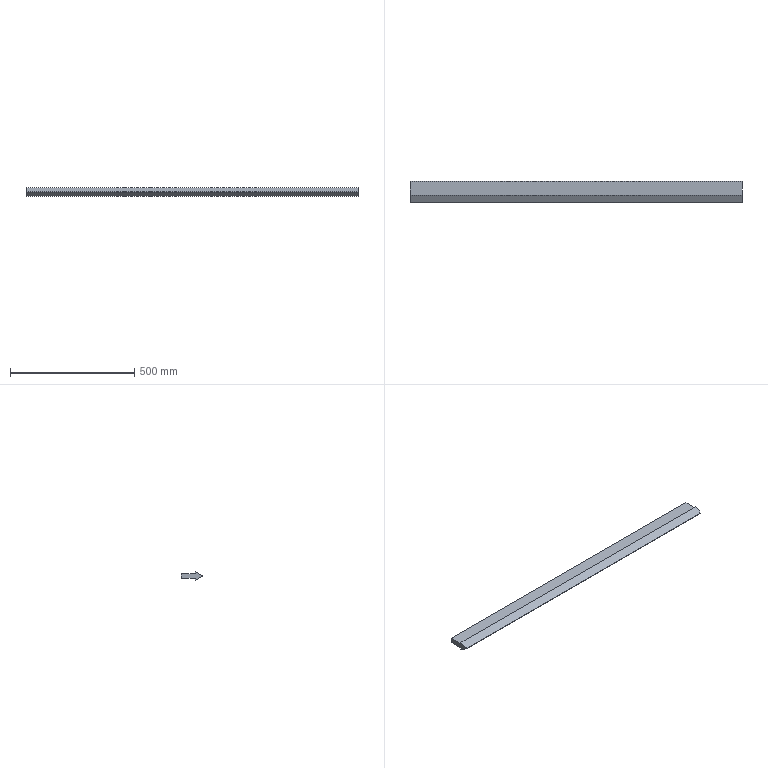Part | SolidWorks | features Extrusion 1, Fillet 1, HoleWzd 1 | 1 solid | 34 faces | box 1337 x 85 x 34.641 mm | volume 2189424 mm3 | cylinder 13 | cone 12 | plane 9 | commonest cylinder face diameters 5 x12 2 x1
STEP:
#1=CARTESIAN_POINT('',(20.,71.,-2.5));
#2=VERTEX_POINT('',#1);
#3=CARTESIAN_POINT('',(20.,71.,2.5));
#4=VERTEX_POINT('',#3);
#5=CARTESIAN_POINT('',(20.,71.,0.));
#6=DIRECTION('',(0.,1.,0.));
#7=DIRECTION('',(0.,0.,1.));
#8=AXIS2_PLACEMENT_3D('',#5,#6,#7);
#9=CIRCLE('',#8,2.5);
#10=EDGE_CURVE('',#2,#4,#9,.T.);
#11=ORIENTED_EDGE('',*,*,#10,.F.);
#12=CARTESIAN_POINT('',(20.,86.,-2.5));
#13=VERTEX_POINT('',#12);
#14=CARTESIAN_POINT('',(20.,86.,-2.5));
#15=DIRECTION('',(0.,1.,0.));
#16=VECTOR('',#15,1000.);
#17=LINE('',#14,#16);
#18=EDGE_CURVE('',#2,#13,#17,.T.);
#19=ORIENTED_EDGE('',*,*,#18,.T.);
#20=CARTESIAN_POINT('',(20.,86.,2.5));
#21=VERTEX_POINT('',#20);
#22=CARTESIAN_POINT('',(20.,86.,0.));
#23=DIRECTION('',(0.,1.,0.));
#24=DIRECTION('',(0.,0.,1.));
#25=AXIS2_PLACEMENT_3D('',#22,#23,#24);
#26=CIRCLE('',#25,2.5);
#27=EDGE_CURVE('',#13,#21,#26,.T.);
#28=ORIENTED_EDGE('',*,*,#27,.T.);
#29=CARTESIAN_POINT('',(20.,86.,2.5));
#30=DIRECTION('',(0.,1.,0.));
#31=VECTOR('',#30,1000.);
#32=LINE('',#29,#31);
#33=EDGE_CURVE('',#4,#21,#32,.T.);
#34=ORIENTED_EDGE('',*,*,#33,.F.);
#35=EDGE_LOOP('',(#11,#19,#28,#34));
#36=FACE_OUTER_BOUND('',#35,.T.);
#37=CARTESIAN_POINT('',(20.,86.,0.));
#38=DIRECTION('',(0.,1.,0.));
#39=DIRECTION('',(0.,0.,1.));
#40=AXIS2_PLACEMENT_3D('',#37,#38,#39);
#41=CYLINDRICAL_SURFACE('',#40,2.5);
#42=ADVANCED_FACE('',(#36),#41,.F.);
#43=CARTESIAN_POINT('',(20.,69.498,0.));
#44=VERTEX_POINT('',#43);
#45=CARTESIAN_POINT('',(20.,71.,2.5));
#46=DIRECTION('',(0.,0.515,0.8572));
#47=VECTOR('',#46,1000.);
#48=LINE('',#45,#47);
#49=EDGE_CURVE('',#44,#4,#48,.T.);
#50=ORIENTED_EDGE('',*,*,#49,.F.);
#51=CARTESIAN_POINT('',(20.,71.,-2.5));
#52=DIRECTION('',(0.,0.515,-0.8572));
#53=VECTOR('',#52,1000.);
#54=LINE('',#51,#53);
#55=EDGE_CURVE('',#44,#2,#54,.T.);
#56=ORIENTED_EDGE('',*,*,#55,.T.);
#57=ORIENTED_EDGE('',*,*,#10,.T.);
#58=EDGE_LOOP('',(#50,#56,#57));
#59=FACE_OUTER_BOUND('',#58,.T.);
#60=CARTESIAN_POINT('',(20.,71.,0.));
#61=DIRECTION('',(0.,1.,0.));
#62=DIRECTION('',(0.,0.,1.));
#63=AXIS2_PLACEMENT_3D('',#60,#61,#62);
#64=CONICAL_SURFACE('',#63,2.5,1.03);
#65=ADVANCED_FACE('',(#59),#64,.F.);
#66=CARTESIAN_POINT('',(45.,71.,-2.5));
#67=VERTEX_POINT('',#66);
#68=CARTESIAN_POINT('',(45.,71.,2.5));
#69=VERTEX_POINT('',#68);
#70=CARTESIAN_POINT('',(45.,71.,0.));
#71=DIRECTION('',(0.,1.,0.));
#72=DIRECTION('',(0.,0.,1.));
#73=AXIS2_PLACEMENT_3D('',#70,#71,#72);
#74=CIRCLE('',#73,2.5);
#75=EDGE_CURVE('',#67,#69,#74,.T.);
#76=ORIENTED_EDGE('',*,*,#75,.F.);
#77=CARTESIAN_POINT('',(45.,86.,-2.5));
#78=VERTEX_POINT('',#77);
#79=CARTESIAN_POINT('',(45.,86.,-2.5));
#80=DIRECTION('',(0.,1.,0.));
#81=VECTOR('',#80,1000.);
#82=LINE('',#79,#81);
#83=EDGE_CURVE('',#67,#78,#82,.T.);
#84=ORIENTED_EDGE('',*,*,#83,.T.);
#85=CARTESIAN_POINT('',(45.,86.,2.5));
#86=VERTEX_POINT('',#85);
#87=CARTESIAN_POINT('',(45.,86.,0.));
#88=DIRECTION('',(0.,1.,0.));
#89=DIRECTION('',(0.,0.,1.));
#90=AXIS2_PLACEMENT_3D('',#87,#88,#89);
#91=CIRCLE('',#90,2.5);
#92=EDGE_CURVE('',#78,#86,#91,.T.);
#93=ORIENTED_EDGE('',*,*,#92,.T.);
#94=CARTESIAN_POINT('',(45.,86.,2.5));
#95=DIRECTION('',(0.,1.,0.));
#96=VECTOR('',#95,1000.);
#97=LINE('',#94,#96);
#98=EDGE_CURVE('',#69,#86,#97,.T.);
#99=ORIENTED_EDGE('',*,*,#98,.F.);
#100=EDGE_LOOP('',(#76,#84,#93,#99));
#101=FACE_OUTER_BOUND('',#100,.T.);
#102=CARTESIAN_POINT('',(45.,86.,0.));
#103=DIRECTION('',(0.,1.,0.));
#104=DIRECTION('',(0.,0.,1.));
#105=AXIS2_PLACEMENT_3D('',#102,#103,#104);
#106=CYLINDRICAL_SURFACE('',#105,2.5);
#107=ADVANCED_FACE('',(#101),#106,.F.);
#108=CARTESIAN_POINT('',(45.,69.498,0.));
#109=VERTEX_POINT('',#108);
#110=CARTESIAN_POINT('',(45.,71.,2.5));
#111=DIRECTION('',(0.,0.515,0.8572));
#112=VECTOR('',#111,1000.);
#113=LINE('',#110,#112);
#114=EDGE_CURVE('',#109,#69,#113,.T.);
#115=ORIENTED_EDGE('',*,*,#114,.F.);
#116=CARTESIAN_POINT('',(45.,71.,-2.5));
#117=DIRECTION('',(0.,0.515,-0.8572));
#118=VECTOR('',#117,1000.);
#119=LINE('',#116,#118);
#120=EDGE_CURVE('',#109,#67,#119,.T.);
#121=ORIENTED_EDGE('',*,*,#120,.T.);
#122=ORIENTED_EDGE('',*,*,#75,.T.);
#123=EDGE_LOOP('',(#115,#121,#122));
#124=FACE_OUTER_BOUND('',#123,.T.);
#125=CARTESIAN_POINT('',(45.,71.,0.));
#126=DIRECTION('',(0.,1.,0.));
#127=DIRECTION('',(0.,0.,1.));
#128=AXIS2_PLACEMENT_3D('',#125,#126,#127);
#129=CONICAL_SURFACE('',#128,2.5,1.03);
#130=ADVANCED_FACE('',(#124),#129,.F.);
#131=CARTESIAN_POINT('',(70.,71.,-2.5));
#132=VERTEX_POINT('',#131);
#133=CARTESIAN_POINT('',(70.,71.,2.5));
#134=VERTEX_POINT('',#133);
#135=CARTESIAN_POINT('',(70.,71.,0.));
#136=DIRECTION('',(0.,1.,0.));
#137=DIRECTION('',(0.,0.,1.));
#138=AXIS2_PLACEMENT_3D('',#135,#136,#137);
#139=CIRCLE('',#138,2.5);
#140=EDGE_CURVE('',#132,#134,#139,.T.);
#141=ORIENTED_EDGE('',*,*,#140,.F.);
#142=CARTESIAN_POINT('',(70.,86.,-2.5));
#143=VERTEX_POINT('',#142);
#144=CARTESIAN_POINT('',(70.,86.,-2.5));
#145=DIRECTION('',(0.,1.,0.));
#146=VECTOR('',#145,1000.);
#147=LINE('',#144,#146);
#148=EDGE_CURVE('',#132,#143,#147,.T.);
#149=ORIENTED_EDGE('',*,*,#148,.T.);
#150=CARTESIAN_POINT('',(70.,86.,2.5));
#151=VERTEX_POINT('',#150);
#152=CARTESIAN_POINT('',(70.,86.,0.));
#153=DIRECTION('',(0.,1.,0.));
#154=DIRECTION('',(0.,0.,1.));
#155=AXIS2_PLACEMENT_3D('',#152,#153,#154);
#156=CIRCLE('',#155,2.5);
#157=EDGE_CURVE('',#143,#151,#156,.T.);
#158=ORIENTED_EDGE('',*,*,#157,.T.);
#159=CARTESIAN_POINT('',(70.,86.,2.5));
#160=DIRECTION('',(0.,1.,0.));
#161=VECTOR('',#160,1000.);
#162=LINE('',#159,#161);
#163=EDGE_CURVE('',#134,#151,#162,.T.);
#164=ORIENTED_EDGE('',*,*,#163,.F.);
#165=EDGE_LOOP('',(#141,#149,#158,#164));
#166=FACE_OUTER_BOUND('',#165,.T.);
#167=CARTESIAN_POINT('',(70.,86.,0.));
#168=DIRECTION('',(0.,1.,0.));
#169=DIRECTION('',(0.,0.,1.));
#170=AXIS2_PLACEMENT_3D('',#167,#168,#169);
#171=CYLINDRICAL_SURFACE('',#170,2.5);
#172=ADVANCED_FACE('',(#166),#171,.F.);
#173=CARTESIAN_POINT('',(70.,69.498,0.));
#174=VERTEX_POINT('',#173);
#175=CARTESIAN_POINT('',(70.,71.,2.5));
#176=DIRECTION('',(0.,0.515,0.8572));
#177=VECTOR('',#176,1000.);
#178=LINE('',#175,#177);
#179=EDGE_CURVE('',#174,#134,#178,.T.);
#180=ORIENTED_EDGE('',*,*,#179,.F.);
#181=CARTESIAN_POINT('',(70.,71.,-2.5));
#182=DIRECTION('',(0.,0.515,-0.8572));
#183=VECTOR('',#182,1000.);
#184=LINE('',#181,#183);
#185=EDGE_CURVE('',#174,#132,#184,.T.);
#186=ORIENTED_EDGE('',*,*,#185,.T.);
#187=ORIENTED_EDGE('',*,*,#140,.T.);
#188=EDGE_LOOP('',(#180,#186,#187));
#189=FACE_OUTER_BOUND('',#188,.T.);
#190=CARTESIAN_POINT('',(70.,71.,0.));
#191=DIRECTION('',(0.,1.,0.));
#192=DIRECTION('',(0.,0.,1.));
#193=AXIS2_PLACEMENT_3D('',#190,#191,#192);
#194=CONICAL_SURFACE('',#193,2.5,1.03);
#195=ADVANCED_FACE('',(#189),#194,.F.);
#196=CARTESIAN_POINT('',(1317.,71.,-2.5));
#197=VERTEX_POINT('',#196);
#198=CARTESIAN_POINT('',(1317.,71.,2.5));
#199=VERTEX_POINT('',#198);
#200=CARTESIAN_POINT('',(1317.,71.,0.));
#201=DIRECTION('',(0.,1.,0.));
#202=DIRECTION('',(0.,0.,1.));
#203=AXIS2_PLACEMENT_3D('',#200,#201,#202);
#204=CIRCLE('',#203,2.5);
#205=EDGE_CURVE('',#197,#199,#204,.T.);
#206=ORIENTED_EDGE('',*,*,#205,.F.);
#207=CARTESIAN_POINT('',(1317.,86.,-2.5));
#208=VERTEX_POINT('',#207);
#209=CARTESIAN_POINT('',(1317.,86.,-2.5));
#210=DIRECTION('',(0.,1.,0.));
#211=VECTOR('',#210,1000.);
#212=LINE('',#209,#211);
#213=EDGE_CURVE('',#197,#208,#212,.T.);
#214=ORIENTED_EDGE('',*,*,#213,.T.);
#215=CARTESIAN_POINT('',(1317.,86.,2.5));
#216=VERTEX_POINT('',#215);
#217=CARTESIAN_POINT('',(1317.,86.,0.));
#218=DIRECTION('',(0.,1.,0.));
#219=DIRECTION('',(0.,0.,1.));
#220=AXIS2_PLACEMENT_3D('',#217,#218,#219);
#221=CIRCLE('',#220,2.5);
#222=EDGE_CURVE('',#208,#216,#221,.T.);
#223=ORIENTED_EDGE('',*,*,#222,.T.);
#224=CARTESIAN_POINT('',(1317.,86.,2.5));
#225=DIRECTION('',(0.,1.,0.));
#226=VECTOR('',#225,1000.);
#227=LINE('',#224,#226);
#228=EDGE_CURVE('',#199,#216,#227,.T.);
#229=ORIENTED_EDGE('',*,*,#228,.F.);
#230=EDGE_LOOP('',(#206,#214,#223,#229));
#231=FACE_OUTER_BOUND('',#230,.T.);
#232=CARTESIAN_POINT('',(1317.,86.,0.));
#233=DIRECTION('',(0.,1.,0.));
#234=DIRECTION('',(0.,0.,1.));
#235=AXIS2_PLACEMENT_3D('',#232,#233,#234);
#236=CYLINDRICAL_SURFACE('',#235,2.5);
#237=ADVANCED_FACE('',(#231),#236,.F.);
#238=CARTESIAN_POINT('',(1317.,69.498,0.));
#239=VERTEX_POINT('',#238);
#240=CARTESIAN_POINT('',(1317.,71.,2.5));
#241=DIRECTION('',(0.,0.515,0.8572));
#242=VECTOR('',#241,1000.);
#243=LINE('',#240,#242);
#244=EDGE_CURVE('',#239,#199,#243,.T.);
#245=ORIENTED_EDGE('',*,*,#244,.F.);
#246=CARTESIAN_POINT('',(1317.,71.,-2.5));
#247=DIRECTION('',(0.,0.515,-0.8572));
#248=VECTOR('',#247,1000.);
#249=LINE('',#246,#248);
#250=EDGE_CURVE('',#239,#197,#249,.T.);
#251=ORIENTED_EDGE('',*,*,#250,.T.);
#252=ORIENTED_EDGE('',*,*,#205,.T.);
#253=EDGE_LOOP('',(#245,#251,#252));
#254=FACE_OUTER_BOUND('',#253,.T.);
#255=CARTESIAN_POINT('',(1317.,71.,0.));
#256=DIRECTION('',(0.,1.,0.));
#257=DIRECTION('',(0.,0.,1.));
#258=AXIS2_PLACEMENT_3D('',#255,#256,#257);
#259=CONICAL_SURFACE('',#258,2.5,1.03);
#260=ADVANCED_FACE('',(#254),#259,.F.);
#261=CARTESIAN_POINT('',(1292.,71.,-2.5));
#262=VERTEX_POINT('',#261);
#263=CARTESIAN_POINT('',(1292.,71.,2.5));
#264=VERTEX_POINT('',#263);
#265=CARTESIAN_POINT('',(1292.,71.,0.));
#266=DIRECTION('',(0.,1.,0.));
#267=DIRECTION('',(0.,0.,1.));
#268=AXIS2_PLACEMENT_3D('',#265,#266,#267);
#269=CIRCLE('',#268,2.5);
#270=EDGE_CURVE('',#262,#264,#269,.T.);
#271=ORIENTED_EDGE('',*,*,#270,.F.);
#272=CARTESIAN_POINT('',(1292.,86.,-2.5));
#273=VERTEX_POINT('',#272);
#274=CARTESIAN_POINT('',(1292.,86.,-2.5));
#275=DIRECTION('',(0.,1.,0.));
#276=VECTOR('',#275,1000.);
#277=LINE('',#274,#276);
#278=EDGE_CURVE('',#262,#273,#277,.T.);
#279=ORIENTED_EDGE('',*,*,#278,.T.);
#280=CARTESIAN_POINT('',(1292.,86.,2.5));
#281=VERTEX_POINT('',#280);
#282=CARTESIAN_POINT('',(1292.,86.,0.));
#283=DIRECTION('',(0.,1.,0.));
#284=DIRECTION('',(0.,0.,1.));
#285=AXIS2_PLACEMENT_3D('',#282,#283,#284);
#286=CIRCLE('',#285,2.5);
#287=EDGE_CURVE('',#273,#281,#286,.T.);
#288=ORIENTED_EDGE('',*,*,#287,.T.);
#289=CARTESIAN_POINT('',(1292.,86.,2.5));
#290=DIRECTION('',(0.,1.,0.));
#291=VECTOR('',#290,1000.);
#292=LINE('',#289,#291);
#293=EDGE_CURVE('',#264,#281,#292,.T.);
#294=ORIENTED_EDGE('',*,*,#293,.F.);
#295=EDGE_LOOP('',(#271,#279,#288,#294));
#296=FACE_OUTER_BOUND('',#295,.T.);
#297=CARTESIAN_POINT('',(1292.,86.,0.));
#298=DIRECTION('',(0.,1.,0.));
#299=DIRECTION('',(0.,0.,1.));
#300=AXIS2_PLACEMENT_3D('',#297,#298,#299);
#301=CYLINDRICAL_SURFACE('',#300,2.5);
#302=ADVANCED_FACE('',(#296),#301,.F.);
#303=CARTESIAN_POINT('',(1292.,69.498,0.));
#304=VERTEX_POINT('',#303);
#305=CARTESIAN_POINT('',(1292.,71.,2.5));
#306=DIRECTION('',(0.,0.515,0.8572));
#307=VECTOR('',#306,1000.);
#308=LINE('',#305,#307);
#309=EDGE_CURVE('',#304,#264,#308,.T.);
#310=ORIENTED_EDGE('',*,*,#309,.F.);
#311=CARTESIAN_POINT('',(1292.,71.,-2.5));
#312=DIRECTION('',(0.,0.515,-0.8572));
#313=VECTOR('',#312,1000.);
#314=LINE('',#311,#313);
#315=EDGE_CURVE('',#304,#262,#314,.T.);
#316=ORIENTED_EDGE('',*,*,#315,.T.);
#317=ORIENTED_EDGE('',*,*,#270,.T.);
#318=EDGE_LOOP('',(#310,#316,#317));
#319=FACE_OUTER_BOUND('',#318,.T.);
#320=CARTESIAN_POINT('',(1292.,71.,0.));
#321=DIRECTION('',(0.,1.,0.));
#322=DIRECTION('',(0.,0.,1.));
#323=AXIS2_PLACEMENT_3D('',#320,#321,#322);
#324=CONICAL_SURFACE('',#323,2.5,1.03);
#325=ADVANCED_FACE('',(#319),#324,.F.);
#326=CARTESIAN_POINT('',(1267.,71.,-2.5));
#327=VERTEX_POINT('',#326);
#328=CARTESIAN_POINT('',(1267.,71.,2.5));
#329=VERTEX_POINT('',#328);
#330=CARTESIAN_POINT('',(1267.,71.,0.));
#331=DIRECTION('',(0.,1.,0.));
#332=DIRECTION('',(0.,0.,1.));
#333=AXIS2_PLACEMENT_3D('',#330,#331,#332);
#334=CIRCLE('',#333,2.5);
#335=EDGE_CURVE('',#327,#329,#334,.T.);
#336=ORIENTED_EDGE('',*,*,#335,.F.);
#337=CARTESIAN_POINT('',(1267.,86.,-2.5));
#338=VERTEX_POINT('',#337);
#339=CARTESIAN_POINT('',(1267.,86.,-2.5));
#340=DIRECTION('',(0.,1.,0.));
#341=VECTOR('',#340,1000.);
#342=LINE('',#339,#341);
#343=EDGE_CURVE('',#327,#338,#342,.T.);
#344=ORIENTED_EDGE('',*,*,#343,.T.);
#345=CARTESIAN_POINT('',(1267.,86.,2.5));
#346=VERTEX_POINT('',#345);
#347=CARTESIAN_POINT('',(1267.,86.,0.));
#348=DIRECTION('',(0.,1.,0.));
#349=DIRECTION('',(0.,0.,1.));
#350=AXIS2_PLACEMENT_3D('',#347,#348,#349);
#351=CIRCLE('',#350,2.5);
#352=EDGE_CURVE('',#338,#346,#351,.T.);
#353=ORIENTED_EDGE('',*,*,#352,.T.);
#354=CARTESIAN_POINT('',(1267.,86.,2.5));
#355=DIRECTION('',(0.,1.,0.));
#356=VECTOR('',#355,1000.);
#357=LINE('',#354,#356);
#358=EDGE_CURVE('',#329,#346,#357,.T.);
#359=ORIENTED_EDGE('',*,*,#358,.F.);
#360=EDGE_LOOP('',(#336,#344,#353,#359));
#361=FACE_OUTER_BOUND('',#360,.T.);
#362=CARTESIAN_POINT('',(1267.,86.,0.));
#363=DIRECTION('',(0.,1.,0.));
#364=DIRECTION('',(0.,0.,1.));
#365=AXIS2_PLACEMENT_3D('',#362,#363,#364);
#366=CYLINDRICAL_SURFACE('',#365,2.5);
#367=ADVANCED_FACE('',(#361),#366,.F.);
#368=CARTESIAN_POINT('',(1267.,69.498,0.));
#369=VERTEX_POINT('',#368);
#370=CARTESIAN_POINT('',(1267.,71.,2.5));
#371=DIRECTION('',(0.,0.515,0.8572));
#372=VECTOR('',#371,1000.);
#373=LINE('',#370,#372);
#374=EDGE_CURVE('',#369,#329,#373,.T.);
#375=ORIENTED_EDGE('',*,*,#374,.F.);
#376=CARTESIAN_POINT('',(1267.,71.,-2.5));
#377=DIRECTION('',(0.,0.515,-0.8572));
#378=VECTOR('',#377,1000.);
#379=LINE('',#376,#378);
#380=EDGE_CURVE('',#369,#327,#379,.T.);
#381=ORIENTED_EDGE('',*,*,#380,.T.);
#382=ORIENTED_EDGE('',*,*,#335,.T.);
#383=EDGE_LOOP('',(#375,#381,#382));
#384=FACE_OUTER_BOUND('',#383,.T.);
#385=CARTESIAN_POINT('',(1267.,71.,0.));
#386=DIRECTION('',(0.,1.,0.));
#387=DIRECTION('',(0.,0.,1.));
#388=AXIS2_PLACEMENT_3D('',#385,#386,#387);
#389=CONICAL_SURFACE('',#388,2.5,1.03);
#390=ADVANCED_FACE('',(#384),#389,.F.);
#391=CARTESIAN_POINT('',(1337.,1.5,-0.866));
#392=VERTEX_POINT('',#391);
#393=CARTESIAN_POINT('',(1337.,30.,-17.321));
#394=VERTEX_POINT('',#393);
#395=CARTESIAN_POINT('',(1337.,0.,0.));
#396=DIRECTION('',(0.,0.866,-0.5));
#397=VECTOR('',#396,1000.);
#398=LINE('',#395,#397);
#399=EDGE_CURVE('',#392,#394,#398,.T.);
#400=ORIENTED_EDGE('',*,*,#399,.F.);
#401=CARTESIAN_POINT('',(0.,1.5,-0.866));
#402=VERTEX_POINT('',#401);
#403=CARTESIAN_POINT('',(1337.,1.5,-0.866));
#404=DIRECTION('',(-1.,0.,0.));
#405=VECTOR('',#404,1000.);
#406=LINE('',#403,#405);
#407=EDGE_CURVE('',#392,#402,#406,.T.);
#408=ORIENTED_EDGE('',*,*,#407,.T.);
#409=CARTESIAN_POINT('',(0.,30.,-17.321));
#410=VERTEX_POINT('',#409);
#411=CARTESIAN_POINT('',(0.,0.,0.));
#412=DIRECTION('',(0.,0.866,-0.5));
#413=VECTOR('',#412,1000.);
#414=LINE('',#411,#413);
#415=EDGE_CURVE('',#402,#410,#414,.T.);
#416=ORIENTED_EDGE('',*,*,#415,.T.);
#417=CARTESIAN_POINT('',(1337.,30.,-17.321));
#418=DIRECTION('',(-1.,0.,0.));
#419=VECTOR('',#418,1000.);
#420=LINE('',#417,#419);
#421=EDGE_CURVE('',#394,#410,#420,.T.);
#422=ORIENTED_EDGE('',*,*,#421,.F.);
#423=EDGE_LOOP('',(#400,#408,#416,#422));
#424=FACE_OUTER_BOUND('',#423,.T.);
#425=CARTESIAN_POINT('',(1337.,0.,0.));
#426=DIRECTION('',(0.,0.5,0.866));
#427=DIRECTION('',(0.,-0.866,0.5));
#428=AXIS2_PLACEMENT_3D('',#425,#426,#427);
#429=PLANE('',#428);
#430=ADVANCED_FACE('',(#424),#429,.F.);
#431=CARTESIAN_POINT('',(0.,30.,-10.));
#432=VERTEX_POINT('',#431);
#433=CARTESIAN_POINT('',(0.,30.,-17.321));
#434=DIRECTION('',(0.,0.,1.));
#435=VECTOR('',#434,1000.);
#436=LINE('',#433,#435);
#437=EDGE_CURVE('',#410,#432,#436,.T.);
#438=ORIENTED_EDGE('',*,*,#437,.T.);
#439=CARTESIAN_POINT('',(1337.,30.,-10.));
#440=VERTEX_POINT('',#439);
#441=CARTESIAN_POINT('',(1337.,30.,-10.));
#442=DIRECTION('',(-1.,0.,0.));
#443=VECTOR('',#442,1000.);
#444=LINE('',#441,#443);
#445=EDGE_CURVE('',#440,#432,#444,.T.);
#446=ORIENTED_EDGE('',*,*,#445,.F.);
#447=CARTESIAN_POINT('',(1337.,30.,-17.321));
#448=DIRECTION('',(0.,0.,1.));
#449=VECTOR('',#448,1000.);
#450=LINE('',#447,#449);
#451=EDGE_CURVE('',#394,#440,#450,.T.);
#452=ORIENTED_EDGE('',*,*,#451,.F.);
#453=ORIENTED_EDGE('',*,*,#421,.T.);
#454=EDGE_LOOP('',(#438,#446,#452,#453));
#455=FACE_OUTER_BOUND('',#454,.T.);
#456=CARTESIAN_POINT('',(1337.,30.,-17.321));
#457=DIRECTION('',(0.,-1.,0.));
#458=DIRECTION('',(0.,0.,-1.));
#459=AXIS2_PLACEMENT_3D('',#456,#457,#458);
#460=PLANE('',#459);
#461=ADVANCED_FACE('',(#455),#460,.F.);
#462=CARTESIAN_POINT('',(0.,86.,-10.));
#463=VERTEX_POINT('',#462);
#464=CARTESIAN_POINT('',(0.,30.,-10.));
#465=DIRECTION('',(0.,1.,0.));
#466=VECTOR('',#465,1000.);
#467=LINE('',#464,#466);
#468=EDGE_CURVE('',#432,#463,#467,.T.);
#469=ORIENTED_EDGE('',*,*,#468,.T.);
#470=CARTESIAN_POINT('',(1337.,86.,-10.));
#471=VERTEX_POINT('',#470);
#472=CARTESIAN_POINT('',(1337.,86.,-10.));
#473=DIRECTION('',(-1.,0.,0.));
#474=VECTOR('',#473,1000.);
#475=LINE('',#472,#474);
#476=EDGE_CURVE('',#471,#463,#475,.T.);
#477=ORIENTED_EDGE('',*,*,#476,.F.);
#478=CARTESIAN_POINT('',(1337.,30.,-10.));
#479=DIRECTION('',(0.,1.,0.));
#480=VECTOR('',#479,1000.);
#481=LINE('',#478,#480);
#482=EDGE_CURVE('',#440,#471,#481,.T.);
#483=ORIENTED_EDGE('',*,*,#482,.F.);
#484=ORIENTED_EDGE('',*,*,#445,.T.);
#485=EDGE_LOOP('',(#469,#477,#483,#484));
#486=FACE_OUTER_BOUND('',#485,.T.);
#487=CARTESIAN_POINT('',(1337.,30.,-10.));
#488=DIRECTION('',(0.,0.,1.));
#489=DIRECTION('',(1.,0.,0.));
#490=AXIS2_PLACEMENT_3D('',#487,#488,#489);
#491=PLANE('',#490);
#492=ADVANCED_FACE('',(#486),#491,.F.);
#493=CARTESIAN_POINT('',(20.,86.,0.));
#494=DIRECTION('',(0.,1.,0.));
#495=DIRECTION('',(0.,0.,1.));
#496=AXIS2_PLACEMENT_3D('',#493,#494,#495);
#497=CIRCLE('',#496,2.5);
#498=EDGE_CURVE('',#21,#13,#497,.T.);
#499=ORIENTED_EDGE('',*,*,#498,.F.);
#500=ORIENTED_EDGE('',*,*,#27,.F.);
#501=EDGE_LOOP('',(#499,#500));
#502=FACE_BOUND('',#501,.T.);
#503=CARTESIAN_POINT('',(45.,86.,0.));
#504=DIRECTION('',(0.,1.,0.));
#505=DIRECTION('',(0.,0.,1.));
#506=AXIS2_PLACEMENT_3D('',#503,#504,#505);
#507=CIRCLE('',#506,2.5);
#508=EDGE_CURVE('',#86,#78,#507,.T.);
#509=ORIENTED_EDGE('',*,*,#508,.F.);
#510=ORIENTED_EDGE('',*,*,#92,.F.);
#511=EDGE_LOOP('',(#509,#510));
#512=FACE_BOUND('',#511,.T.);
#513=CARTESIAN_POINT('',(70.,86.,0.));
#514=DIRECTION('',(0.,1.,0.));
#515=DIRECTION('',(0.,0.,1.));
#516=AXIS2_PLACEMENT_3D('',#513,#514,#515);
#517=CIRCLE('',#516,2.5);
#518=EDGE_CURVE('',#151,#143,#517,.T.);
#519=ORIENTED_EDGE('',*,*,#518,.F.);
#520=ORIENTED_EDGE('',*,*,#157,.F.);
#521=EDGE_LOOP('',(#519,#520));
#522=FACE_BOUND('',#521,.T.);
#523=CARTESIAN_POINT('',(1317.,86.,0.));
#524=DIRECTION('',(0.,1.,0.));
#525=DIRECTION('',(0.,0.,1.));
#526=AXIS2_PLACEMENT_3D('',#523,#524,#525);
#527=CIRCLE('',#526,2.5);
#528=EDGE_CURVE('',#216,#208,#527,.T.);
#529=ORIENTED_EDGE('',*,*,#528,.F.);
#530=ORIENTED_EDGE('',*,*,#222,.F.);
#531=EDGE_LOOP('',(#529,#530));
#532=FACE_BOUND('',#531,.T.);
#533=CARTESIAN_POINT('',(1292.,86.,0.));
#534=DIRECTION('',(0.,1.,0.));
#535=DIRECTION('',(0.,0.,1.));
#536=AXIS2_PLACEMENT_3D('',#533,#534,#535);
#537=CIRCLE('',#536,2.5);
#538=EDGE_CURVE('',#281,#273,#537,.T.);
#539=ORIENTED_EDGE('',*,*,#538,.F.);
#540=ORIENTED_EDGE('',*,*,#287,.F.);
#541=EDGE_LOOP('',(#539,#540));
#542=FACE_BOUND('',#541,.T.);
#543=CARTESIAN_POINT('',(1267.,86.,0.));
#544=DIRECTION('',(0.,1.,0.));
#545=DIRECTION('',(0.,0.,1.));
#546=AXIS2_PLACEMENT_3D('',#543,#544,#545);
#547=CIRCLE('',#546,2.5);
#548=EDGE_CURVE('',#346,#338,#547,.T.);
#549=ORIENTED_EDGE('',*,*,#548,.F.);
#550=ORIENTED_EDGE('',*,*,#352,.F.);
#551=EDGE_LOOP('',(#549,#550));
#552=FACE_BOUND('',#551,.T.);
#553=CARTESIAN_POINT('',(0.,86.,10.));
#554=VERTEX_POINT('',#553);
#555=CARTESIAN_POINT('',(0.,86.,-10.));
#556=DIRECTION('',(0.,0.,1.));
#557=VECTOR('',#556,1000.);
#558=LINE('',#555,#557);
#559=EDGE_CURVE('',#463,#554,#558,.T.);
#560=ORIENTED_EDGE('',*,*,#559,.T.);
#561=CARTESIAN_POINT('',(1337.,86.,10.));
#562=VERTEX_POINT('',#561);
#563=CARTESIAN_POINT('',(1337.,86.,10.));
#564=DIRECTION('',(-1.,0.,0.));
#565=VECTOR('',#564,1000.);
#566=LINE('',#563,#565);
#567=EDGE_CURVE('',#562,#554,#566,.T.);
#568=ORIENTED_EDGE('',*,*,#567,.F.);
#569=CARTESIAN_POINT('',(1337.,86.,-10.));
#570=DIRECTION('',(0.,0.,1.));
#571=VECTOR('',#570,1000.);
#572=LINE('',#569,#571);
#573=EDGE_CURVE('',#471,#562,#572,.T.);
#574=ORIENTED_EDGE('',*,*,#573,.F.);
#575=ORIENTED_EDGE('',*,*,#476,.T.);
#576=EDGE_LOOP('',(#560,#568,#574,#575));
#577=FACE_OUTER_BOUND('',#576,.T.);
#578=CARTESIAN_POINT('',(1337.,86.,-10.));
#579=DIRECTION('',(0.,-1.,0.));
#580=DIRECTION('',(0.,0.,-1.));
#581=AXIS2_PLACEMENT_3D('',#578,#579,#580);
#582=PLANE('',#581);
#583=ADVANCED_FACE('',(#502,#512,#522,#532,#542,#552,#577),#582,.F.);
#584=CARTESIAN_POINT('',(0.,30.,10.));
#585=VERTEX_POINT('',#584);
#586=CARTESIAN_POINT('',(0.,86.,10.));
#587=DIRECTION('',(0.,-1.,0.));
#588=VECTOR('',#587,1000.);
#589=LINE('',#586,#588);
#590=EDGE_CURVE('',#554,#585,#589,.T.);
#591=ORIENTED_EDGE('',*,*,#590,.T.);
#592=CARTESIAN_POINT('',(1337.,30.,10.));
#593=VERTEX_POINT('',#592);
#594=CARTESIAN_POINT('',(1337.,30.,10.));
#595=DIRECTION('',(-1.,0.,0.));
#596=VECTOR('',#595,1000.);
#597=LINE('',#594,#596);
#598=EDGE_CURVE('',#593,#585,#597,.T.);
#599=ORIENTED_EDGE('',*,*,#598,.F.);
#600=CARTESIAN_POINT('',(1337.,86.,10.));
#601=DIRECTION('',(0.,-1.,0.));
#602=VECTOR('',#601,1000.);
#603=LINE('',#600,#602);
#604=EDGE_CURVE('',#562,#593,#603,.T.);
#605=ORIENTED_EDGE('',*,*,#604,.F.);
#606=ORIENTED_EDGE('',*,*,#567,.T.);
#607=EDGE_LOOP('',(#591,#599,#605,#606));
#608=FACE_OUTER_BOUND('',#607,.T.);
#609=CARTESIAN_POINT('',(1337.,86.,10.));
#610=DIRECTION('',(0.,0.,-1.));
#611=DIRECTION('',(0.,1.,0.));
#612=AXIS2_PLACEMENT_3D('',#609,#610,#611);
#613=PLANE('',#612);
#614=ADVANCED_FACE('',(#608),#613,.F.);
#615=CARTESIAN_POINT('',(0.,30.,17.321));
#616=VERTEX_POINT('',#615);
#617=CARTESIAN_POINT('',(0.,30.,10.));
#618=DIRECTION('',(0.,0.,1.));
#619=VECTOR('',#618,1000.);
#620=LINE('',#617,#619);
#621=EDGE_CURVE('',#585,#616,#620,.T.);
#622=ORIENTED_EDGE('',*,*,#621,.T.);
#623=CARTESIAN_POINT('',(1337.,30.,17.321));
#624=VERTEX_POINT('',#623);
#625=CARTESIAN_POINT('',(1337.,30.,17.321));
#626=DIRECTION('',(-1.,0.,0.));
#627=VECTOR('',#626,1000.);
#628=LINE('',#625,#627);
#629=EDGE_CURVE('',#624,#616,#628,.T.);
#630=ORIENTED_EDGE('',*,*,#629,.F.);
#631=CARTESIAN_POINT('',(1337.,30.,10.));
#632=DIRECTION('',(0.,0.,1.));
#633=VECTOR('',#632,1000.);
#634=LINE('',#631,#633);
#635=EDGE_CURVE('',#593,#624,#634,.T.);
#636=ORIENTED_EDGE('',*,*,#635,.F.);
#637=ORIENTED_EDGE('',*,*,#598,.T.);
#638=EDGE_LOOP('',(#622,#630,#636,#637));
#639=FACE_OUTER_BOUND('',#638,.T.);
#640=CARTESIAN_POINT('',(1337.,30.,10.));
#641=DIRECTION('',(0.,-1.,0.));
#642=DIRECTION('',(0.,0.,-1.));
#643=AXIS2_PLACEMENT_3D('',#640,#641,#642);
#644=PLANE('',#643);
#645=ADVANCED_FACE('',(#639),#644,.F.);
#646=CARTESIAN_POINT('',(0.,1.5,0.866));
#647=VERTEX_POINT('',#646);
#648=CARTESIAN_POINT('',(0.,0.,0.));
#649=DIRECTION('',(0.,-0.866,-0.5));
#650=VECTOR('',#649,1000.);
#651=LINE('',#648,#650);
#652=EDGE_CURVE('',#616,#647,#651,.T.);
#653=ORIENTED_EDGE('',*,*,#652,.T.);
#654=CARTESIAN_POINT('',(1337.,1.5,0.866));
#655=VERTEX_POINT('',#654);
#656=CARTESIAN_POINT('',(1337.,1.5,0.866));
#657=DIRECTION('',(1.,0.,0.));
#658=VECTOR('',#657,1000.);
#659=LINE('',#656,#658);
#660=EDGE_CURVE('',#647,#655,#659,.T.);
#661=ORIENTED_EDGE('',*,*,#660,.T.);
#662=CARTESIAN_POINT('',(1337.,0.,0.));
#663=DIRECTION('',(0.,-0.866,-0.5));
#664=VECTOR('',#663,1000.);
#665=LINE('',#662,#664);
#666=EDGE_CURVE('',#624,#655,#665,.T.);
#667=ORIENTED_EDGE('',*,*,#666,.F.);
#668=ORIENTED_EDGE('',*,*,#629,.T.);
#669=EDGE_LOOP('',(#653,#661,#667,#668));
#670=FACE_OUTER_BOUND('',#669,.T.);
#671=CARTESIAN_POINT('',(1337.,0.,0.));
#672=DIRECTION('',(0.,0.5,-0.866));
#673=DIRECTION('',(0.,0.866,0.5));
#674=AXIS2_PLACEMENT_3D('',#671,#672,#673);
#675=PLANE('',#674);
#676=ADVANCED_FACE('',(#670),#675,.F.);
#677=ORIENTED_EDGE('',*,*,#666,.T.);
#678=CARTESIAN_POINT('',(1337.,2.,0.));
#679=DIRECTION('',(1.,0.,0.));
#680=DIRECTION('',(0.,0.,-1.));
#681=AXIS2_PLACEMENT_3D('',#678,#679,#680);
#682=CIRCLE('',#681,1.);
#683=EDGE_CURVE('',#655,#392,#682,.T.);
#684=ORIENTED_EDGE('',*,*,#683,.T.);
#685=ORIENTED_EDGE('',*,*,#399,.T.);
#686=ORIENTED_EDGE('',*,*,#451,.T.);
#687=ORIENTED_EDGE('',*,*,#482,.T.);
#688=ORIENTED_EDGE('',*,*,#573,.T.);
#689=ORIENTED_EDGE('',*,*,#604,.T.);
#690=ORIENTED_EDGE('',*,*,#635,.T.);
#691=EDGE_LOOP('',(#677,#684,#685,#686,#687,#688,#689,#690));
#692=FACE_OUTER_BOUND('',#691,.T.);
#693=CARTESIAN_POINT('',(1337.,0.,0.));
#694=DIRECTION('',(1.,0.,0.));
#695=DIRECTION('',(0.,0.,-1.));
#696=AXIS2_PLACEMENT_3D('',#693,#694,#695);
#697=PLANE('',#696);
#698=ADVANCED_FACE('',(#692),#697,.T.);
#699=ORIENTED_EDGE('',*,*,#415,.F.);
#700=CARTESIAN_POINT('',(0.,2.,0.));
#701=DIRECTION('',(-1.,0.,0.));
#702=DIRECTION('',(0.,0.,-1.));
#703=AXIS2_PLACEMENT_3D('',#700,#701,#702);
#704=CIRCLE('',#703,1.);
#705=EDGE_CURVE('',#402,#647,#704,.T.);
#706=ORIENTED_EDGE('',*,*,#705,.T.);
#707=ORIENTED_EDGE('',*,*,#652,.F.);
#708=ORIENTED_EDGE('',*,*,#621,.F.);
#709=ORIENTED_EDGE('',*,*,#590,.F.);
#710=ORIENTED_EDGE('',*,*,#559,.F.);
#711=ORIENTED_EDGE('',*,*,#468,.F.);
#712=ORIENTED_EDGE('',*,*,#437,.F.);
#713=EDGE_LOOP('',(#699,#706,#707,#708,#709,#710,#711,#712));
#714=FACE_OUTER_BOUND('',#713,.T.);
#715=CARTESIAN_POINT('',(0.,0.,0.));
#716=DIRECTION('',(1.,0.,0.));
#717=DIRECTION('',(0.,0.,-1.));
#718=AXIS2_PLACEMENT_3D('',#715,#716,#717);
#719=PLANE('',#718);
#720=ADVANCED_FACE('',(#714),#719,.F.);
#721=ORIENTED_EDGE('',*,*,#683,.F.);
#722=ORIENTED_EDGE('',*,*,#660,.F.);
#723=ORIENTED_EDGE('',*,*,#705,.F.);
#724=ORIENTED_EDGE('',*,*,#407,.F.);
#725=EDGE_LOOP('',(#721,#722,#723,#724));
#726=FACE_OUTER_BOUND('',#725,.T.);
#727=CARTESIAN_POINT('',(1337.,2.,0.));
#728=DIRECTION('',(-1.,0.,0.));
#729=DIRECTION('',(0.,0.,1.));
#730=AXIS2_PLACEMENT_3D('',#727,#728,#729);
#731=CYLINDRICAL_SURFACE('',#730,1.);
#732=ADVANCED_FACE('',(#726),#731,.T.);
#733=ORIENTED_EDGE('',*,*,#380,.F.);
#734=ORIENTED_EDGE('',*,*,#374,.T.);
#735=CARTESIAN_POINT('',(1267.,71.,0.));
#736=DIRECTION('',(0.,1.,0.));
#737=DIRECTION('',(0.,0.,1.));
#738=AXIS2_PLACEMENT_3D('',#735,#736,#737);
#739=CIRCLE('',#738,2.5);
#740=EDGE_CURVE('',#329,#327,#739,.T.);
#741=ORIENTED_EDGE('',*,*,#740,.T.);
#742=EDGE_LOOP('',(#733,#734,#741));
#743=FACE_OUTER_BOUND('',#742,.T.);
#744=CARTESIAN_POINT('',(1267.,71.,0.));
#745=DIRECTION('',(0.,1.,0.));
#746=DIRECTION('',(0.,0.,1.));
#747=AXIS2_PLACEMENT_3D('',#744,#745,#746);
#748=CONICAL_SURFACE('',#747,2.5,1.03);
#749=ADVANCED_FACE('',(#743),#748,.F.);
#750=ORIENTED_EDGE('',*,*,#343,.F.);
#751=ORIENTED_EDGE('',*,*,#740,.F.);
#752=ORIENTED_EDGE('',*,*,#358,.T.);
#753=ORIENTED_EDGE('',*,*,#548,.T.);
#754=EDGE_LOOP('',(#750,#751,#752,#753));
#755=FACE_OUTER_BOUND('',#754,.T.);
#756=CARTESIAN_POINT('',(1267.,86.,0.));
#757=DIRECTION('',(0.,1.,0.));
#758=DIRECTION('',(0.,0.,1.));
#759=AXIS2_PLACEMENT_3D('',#756,#757,#758);
#760=CYLINDRICAL_SURFACE('',#759,2.5);
#761=ADVANCED_FACE('',(#755),#760,.F.);
#762=ORIENTED_EDGE('',*,*,#315,.F.);
#763=ORIENTED_EDGE('',*,*,#309,.T.);
#764=CARTESIAN_POINT('',(1292.,71.,0.));
#765=DIRECTION('',(0.,1.,0.));
#766=DIRECTION('',(0.,0.,1.));
#767=AXIS2_PLACEMENT_3D('',#764,#765,#766);
#768=CIRCLE('',#767,2.5);
#769=EDGE_CURVE('',#264,#262,#768,.T.);
#770=ORIENTED_EDGE('',*,*,#769,.T.);
#771=EDGE_LOOP('',(#762,#763,#770));
#772=FACE_OUTER_BOUND('',#771,.T.);
#773=CARTESIAN_POINT('',(1292.,71.,0.));
#774=DIRECTION('',(0.,1.,0.));
#775=DIRECTION('',(0.,0.,1.));
#776=AXIS2_PLACEMENT_3D('',#773,#774,#775);
#777=CONICAL_SURFACE('',#776,2.5,1.03);
#778=ADVANCED_FACE('',(#772),#777,.F.);
#779=ORIENTED_EDGE('',*,*,#278,.F.);
#780=ORIENTED_EDGE('',*,*,#769,.F.);
#781=ORIENTED_EDGE('',*,*,#293,.T.);
#782=ORIENTED_EDGE('',*,*,#538,.T.);
#783=EDGE_LOOP('',(#779,#780,#781,#782));
#784=FACE_OUTER_BOUND('',#783,.T.);
#785=CARTESIAN_POINT('',(1292.,86.,0.));
#786=DIRECTION('',(0.,1.,0.));
#787=DIRECTION('',(0.,0.,1.));
#788=AXIS2_PLACEMENT_3D('',#785,#786,#787);
#789=CYLINDRICAL_SURFACE('',#788,2.5);
#790=ADVANCED_FACE('',(#784),#789,.F.);
#791=ORIENTED_EDGE('',*,*,#250,.F.);
#792=ORIENTED_EDGE('',*,*,#244,.T.);
#793=CARTESIAN_POINT('',(1317.,71.,0.));
#794=DIRECTION('',(0.,1.,0.));
#795=DIRECTION('',(0.,0.,1.));
#796=AXIS2_PLACEMENT_3D('',#793,#794,#795);
#797=CIRCLE('',#796,2.5);
#798=EDGE_CURVE('',#199,#197,#797,.T.);
#799=ORIENTED_EDGE('',*,*,#798,.T.);
#800=EDGE_LOOP('',(#791,#792,#799));
#801=FACE_OUTER_BOUND('',#800,.T.);
#802=CARTESIAN_POINT('',(1317.,71.,0.));
#803=DIRECTION('',(0.,1.,0.));
#804=DIRECTION('',(0.,0.,1.));
#805=AXIS2_PLACEMENT_3D('',#802,#803,#804);
#806=CONICAL_SURFACE('',#805,2.5,1.03);
#807=ADVANCED_FACE('',(#801),#806,.F.);
#808=ORIENTED_EDGE('',*,*,#213,.F.);
#809=ORIENTED_EDGE('',*,*,#798,.F.);
#810=ORIENTED_EDGE('',*,*,#228,.T.);
#811=ORIENTED_EDGE('',*,*,#528,.T.);
#812=EDGE_LOOP('',(#808,#809,#810,#811));
#813=FACE_OUTER_BOUND('',#812,.T.);
#814=CARTESIAN_POINT('',(1317.,86.,0.));
#815=DIRECTION('',(0.,1.,0.));
#816=DIRECTION('',(0.,0.,1.));
#817=AXIS2_PLACEMENT_3D('',#814,#815,#816);
#818=CYLINDRICAL_SURFACE('',#817,2.5);
#819=ADVANCED_FACE('',(#813),#818,.F.);
#820=ORIENTED_EDGE('',*,*,#185,.F.);
#821=ORIENTED_EDGE('',*,*,#179,.T.);
#822=CARTESIAN_POINT('',(70.,71.,0.));
#823=DIRECTION('',(0.,1.,0.));
#824=DIRECTION('',(0.,0.,1.));
#825=AXIS2_PLACEMENT_3D('',#822,#823,#824);
#826=CIRCLE('',#825,2.5);
#827=EDGE_CURVE('',#134,#132,#826,.T.);
#828=ORIENTED_EDGE('',*,*,#827,.T.);
#829=EDGE_LOOP('',(#820,#821,#828));
#830=FACE_OUTER_BOUND('',#829,.T.);
#831=CARTESIAN_POINT('',(70.,71.,0.));
#832=DIRECTION('',(0.,1.,0.));
#833=DIRECTION('',(0.,0.,1.));
#834=AXIS2_PLACEMENT_3D('',#831,#832,#833);
#835=CONICAL_SURFACE('',#834,2.5,1.03);
#836=ADVANCED_FACE('',(#830),#835,.F.);
#837=ORIENTED_EDGE('',*,*,#148,.F.);
#838=ORIENTED_EDGE('',*,*,#827,.F.);
#839=ORIENTED_EDGE('',*,*,#163,.T.);
#840=ORIENTED_EDGE('',*,*,#518,.T.);
#841=EDGE_LOOP('',(#837,#838,#839,#840));
#842=FACE_OUTER_BOUND('',#841,.T.);
#843=CARTESIAN_POINT('',(70.,86.,0.));
#844=DIRECTION('',(0.,1.,0.));
#845=DIRECTION('',(0.,0.,1.));
#846=AXIS2_PLACEMENT_3D('',#843,#844,#845);
#847=CYLINDRICAL_SURFACE('',#846,2.5);
#848=ADVANCED_FACE('',(#842),#847,.F.);
#849=ORIENTED_EDGE('',*,*,#120,.F.);
#850=ORIENTED_EDGE('',*,*,#114,.T.);
#851=CARTESIAN_POINT('',(45.,71.,0.));
#852=DIRECTION('',(0.,1.,0.));
#853=DIRECTION('',(0.,0.,1.));
#854=AXIS2_PLACEMENT_3D('',#851,#852,#853);
#855=CIRCLE('',#854,2.5);
#856=EDGE_CURVE('',#69,#67,#855,.T.);
#857=ORIENTED_EDGE('',*,*,#856,.T.);
#858=EDGE_LOOP('',(#849,#850,#857));
#859=FACE_OUTER_BOUND('',#858,.T.);
#860=CARTESIAN_POINT('',(45.,71.,0.));
#861=DIRECTION('',(0.,1.,0.));
#862=DIRECTION('',(0.,0.,1.));
#863=AXIS2_PLACEMENT_3D('',#860,#861,#862);
#864=CONICAL_SURFACE('',#863,2.5,1.03);
#865=ADVANCED_FACE('',(#859),#864,.F.);
#866=ORIENTED_EDGE('',*,*,#83,.F.);
#867=ORIENTED_EDGE('',*,*,#856,.F.);
#868=ORIENTED_EDGE('',*,*,#98,.T.);
#869=ORIENTED_EDGE('',*,*,#508,.T.);
#870=EDGE_LOOP('',(#866,#867,#868,#869));
#871=FACE_OUTER_BOUND('',#870,.T.);
#872=CARTESIAN_POINT('',(45.,86.,0.));
#873=DIRECTION('',(0.,1.,0.));
#874=DIRECTION('',(0.,0.,1.));
#875=AXIS2_PLACEMENT_3D('',#872,#873,#874);
#876=CYLINDRICAL_SURFACE('',#875,2.5);
#877=ADVANCED_FACE('',(#871),#876,.F.);
#878=ORIENTED_EDGE('',*,*,#55,.F.);
#879=ORIENTED_EDGE('',*,*,#49,.T.);
#880=CARTESIAN_POINT('',(20.,71.,0.));
#881=DIRECTION('',(0.,1.,0.));
#882=DIRECTION('',(0.,0.,1.));
#883=AXIS2_PLACEMENT_3D('',#880,#881,#882);
#884=CIRCLE('',#883,2.5);
#885=EDGE_CURVE('',#4,#2,#884,.T.);
#886=ORIENTED_EDGE('',*,*,#885,.T.);
#887=EDGE_LOOP('',(#878,#879,#886));
#888=FACE_OUTER_BOUND('',#887,.T.);
#889=CARTESIAN_POINT('',(20.,71.,0.));
#890=DIRECTION('',(0.,1.,0.));
#891=DIRECTION('',(0.,0.,1.));
#892=AXIS2_PLACEMENT_3D('',#889,#890,#891);
#893=CONICAL_SURFACE('',#892,2.5,1.03);
#894=ADVANCED_FACE('',(#888),#893,.F.);
#895=ORIENTED_EDGE('',*,*,#18,.F.);
#896=ORIENTED_EDGE('',*,*,#885,.F.);
#897=ORIENTED_EDGE('',*,*,#33,.T.);
#898=ORIENTED_EDGE('',*,*,#498,.T.);
#899=EDGE_LOOP('',(#895,#896,#897,#898));
#900=FACE_OUTER_BOUND('',#899,.T.);
#901=CARTESIAN_POINT('',(20.,86.,0.));
#902=DIRECTION('',(0.,1.,0.));
#903=DIRECTION('',(0.,0.,1.));
#904=AXIS2_PLACEMENT_3D('',#901,#902,#903);
#905=CYLINDRICAL_SURFACE('',#904,2.5);
#906=ADVANCED_FACE('',(#900),#905,.F.);
#907=CLOSED_SHELL('',(#42,#65,#107,#130,#172,#195,#237,#260,#302,#325,#367,#390,#430,#461,#492,#583,#614,#645,#676,#698,#720,#732,#749,#761,#778,#790,#807,#819,#836,#848,#865,#877,#894,#906));
#908=MANIFOLD_SOLID_BREP('',#907);
#909=CARTESIAN_POINT('',(0.,0.,0.));
#910=DIRECTION('',(0.,0.,1.));
#911=DIRECTION('',(1.,0.,0.));
#912=AXIS2_PLACEMENT_3D('',#909,#910,#911);
#913=(LENGTH_UNIT()NAMED_UNIT(*)SI_UNIT(.MILLI.,.METRE.));
#914=UNCERTAINTY_MEASURE_WITH_UNIT(LENGTH_MEASURE(0.00001),#913,'','');
#915=(NAMED_UNIT(*)PLANE_ANGLE_UNIT()SI_UNIT($,.RADIAN.));
#916=(NAMED_UNIT(*)SI_UNIT($,.STERADIAN.)SOLID_ANGLE_UNIT());
#917=(GEOMETRIC_REPRESENTATION_CONTEXT(3)GLOBAL_UNCERTAINTY_ASSIGNED_CONTEXT((#914))GLOBAL_UNIT_ASSIGNED_CONTEXT((#913,#915,#916))REPRESENTATION_CONTEXT('',''));
#918=ADVANCED_BREP_SHAPE_REPRESENTATION('',(#908,#912),#917);